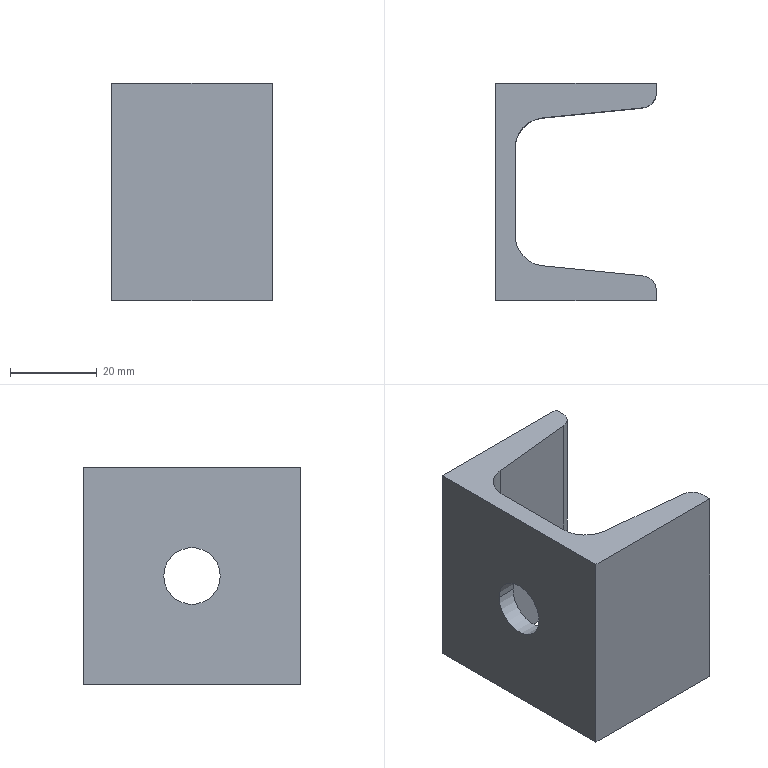Part | SolidWorks | features BaseBody 1 | 1 solid | 16 faces | box 37 x 50 x 50 mm | volume 34025 mm3 | plane 10 | cylinder 6 | commonest cylinder face diameters 7 x2 13 x2 14 x2
STEP:
#1=CARTESIAN_POINT('',(-13.5,-6.5,25.));
#2=VERTEX_POINT('',#1);
#3=CARTESIAN_POINT('',(-13.5,6.5,25.));
#4=VERTEX_POINT('',#3);
#5=CARTESIAN_POINT('',(-13.5,0.,25.));
#6=DIRECTION('',(1.,0.,0.));
#7=DIRECTION('',(0.,1.,0.));
#8=AXIS2_PLACEMENT_3D('',#5,#6,#7);
#9=CIRCLE('',#8,6.5);
#10=EDGE_CURVE('',#2,#4,#9,.T.);
#11=ORIENTED_EDGE('',*,*,#10,.F.);
#12=CARTESIAN_POINT('',(-9.,-6.5,25.));
#13=VERTEX_POINT('',#12);
#14=CARTESIAN_POINT('',(-13.5,-6.5,25.));
#15=DIRECTION('',(1.,0.,0.));
#16=VECTOR('',#15,1000.);
#17=LINE('',#14,#16);
#18=EDGE_CURVE('',#2,#13,#17,.T.);
#19=ORIENTED_EDGE('',*,*,#18,.T.);
#20=CARTESIAN_POINT('',(-9.,6.5,25.));
#21=VERTEX_POINT('',#20);
#22=CARTESIAN_POINT('',(-9.,0.,25.));
#23=DIRECTION('',(-1.,0.,0.));
#24=DIRECTION('',(0.,1.,0.));
#25=AXIS2_PLACEMENT_3D('',#22,#23,#24);
#26=CIRCLE('',#25,6.5);
#27=EDGE_CURVE('',#21,#13,#26,.T.);
#28=ORIENTED_EDGE('',*,*,#27,.F.);
#29=CARTESIAN_POINT('',(-13.5,6.5,25.));
#30=DIRECTION('',(1.,0.,0.));
#31=VECTOR('',#30,1000.);
#32=LINE('',#29,#31);
#33=EDGE_CURVE('',#4,#21,#32,.T.);
#34=ORIENTED_EDGE('',*,*,#33,.F.);
#35=EDGE_LOOP('',(#11,#19,#28,#34));
#36=FACE_OUTER_BOUND('',#35,.T.);
#37=CARTESIAN_POINT('',(-13.5,0.,25.));
#38=DIRECTION('',(1.,0.,0.));
#39=DIRECTION('',(0.,1.,0.));
#40=AXIS2_PLACEMENT_3D('',#37,#38,#39);
#41=CYLINDRICAL_SURFACE('',#40,6.5);
#42=ADVANCED_FACE('',(#36),#41,.F.);
#43=CARTESIAN_POINT('',(-13.5,0.,25.));
#44=DIRECTION('',(1.,0.,0.));
#45=DIRECTION('',(0.,1.,0.));
#46=AXIS2_PLACEMENT_3D('',#43,#44,#45);
#47=CIRCLE('',#46,6.5);
#48=EDGE_CURVE('',#4,#2,#47,.T.);
#49=ORIENTED_EDGE('',*,*,#48,.T.);
#50=ORIENTED_EDGE('',*,*,#10,.T.);
#51=EDGE_LOOP('',(#49,#50));
#52=FACE_BOUND('',#51,.T.);
#53=CARTESIAN_POINT('',(-13.5,25.,0.));
#54=VERTEX_POINT('',#53);
#55=CARTESIAN_POINT('',(-13.5,-25.,0.));
#56=VERTEX_POINT('',#55);
#57=CARTESIAN_POINT('',(-13.5,0.,0.));
#58=DIRECTION('',(0.,-1.,0.));
#59=VECTOR('',#58,1000.);
#60=LINE('',#57,#59);
#61=EDGE_CURVE('',#54,#56,#60,.T.);
#62=ORIENTED_EDGE('',*,*,#61,.T.);
#63=CARTESIAN_POINT('',(-13.5,-25.,50.));
#64=VERTEX_POINT('',#63);
#65=CARTESIAN_POINT('',(-13.5,-25.,0.));
#66=DIRECTION('',(0.,0.,1.));
#67=VECTOR('',#66,1000.);
#68=LINE('',#65,#67);
#69=EDGE_CURVE('',#56,#64,#68,.T.);
#70=ORIENTED_EDGE('',*,*,#69,.T.);
#71=CARTESIAN_POINT('',(-13.5,25.,50.));
#72=VERTEX_POINT('',#71);
#73=CARTESIAN_POINT('',(-13.5,0.,50.));
#74=DIRECTION('',(0.,1.,0.));
#75=VECTOR('',#74,1000.);
#76=LINE('',#73,#75);
#77=EDGE_CURVE('',#64,#72,#76,.T.);
#78=ORIENTED_EDGE('',*,*,#77,.T.);
#79=CARTESIAN_POINT('',(-13.5,25.,0.));
#80=DIRECTION('',(0.,0.,-1.));
#81=VECTOR('',#80,1000.);
#82=LINE('',#79,#81);
#83=EDGE_CURVE('',#72,#54,#82,.T.);
#84=ORIENTED_EDGE('',*,*,#83,.T.);
#85=EDGE_LOOP('',(#62,#70,#78,#84));
#86=FACE_OUTER_BOUND('',#85,.T.);
#87=CARTESIAN_POINT('',(-13.5,0.,0.));
#88=DIRECTION('',(-1.,0.,0.));
#89=DIRECTION('',(0.,-1.,0.));
#90=AXIS2_PLACEMENT_3D('',#87,#88,#89);
#91=PLANE('',#90);
#92=ADVANCED_FACE('',(#52,#86),#91,.T.);
#93=ORIENTED_EDGE('',*,*,#18,.F.);
#94=ORIENTED_EDGE('',*,*,#48,.F.);
#95=ORIENTED_EDGE('',*,*,#33,.T.);
#96=CARTESIAN_POINT('',(-9.,0.,25.));
#97=DIRECTION('',(-1.,0.,0.));
#98=DIRECTION('',(0.,1.,0.));
#99=AXIS2_PLACEMENT_3D('',#96,#97,#98);
#100=CIRCLE('',#99,6.5);
#101=EDGE_CURVE('',#13,#21,#100,.T.);
#102=ORIENTED_EDGE('',*,*,#101,.F.);
#103=EDGE_LOOP('',(#93,#94,#95,#102));
#104=FACE_OUTER_BOUND('',#103,.T.);
#105=CARTESIAN_POINT('',(-13.5,0.,25.));
#106=DIRECTION('',(1.,0.,0.));
#107=DIRECTION('',(0.,1.,0.));
#108=AXIS2_PLACEMENT_3D('',#105,#106,#107);
#109=CYLINDRICAL_SURFACE('',#108,6.5);
#110=ADVANCED_FACE('',(#104),#109,.F.);
#111=CARTESIAN_POINT('',(23.5,-25.,0.));
#112=VERTEX_POINT('',#111);
#113=CARTESIAN_POINT('',(23.5,-25.,0.));
#114=DIRECTION('',(1.,0.,0.));
#115=VECTOR('',#114,1000.);
#116=LINE('',#113,#115);
#117=EDGE_CURVE('',#56,#112,#116,.T.);
#118=ORIENTED_EDGE('',*,*,#117,.T.);
#119=CARTESIAN_POINT('',(23.5,-25.,50.));
#120=VERTEX_POINT('',#119);
#121=CARTESIAN_POINT('',(23.5,-25.,0.));
#122=DIRECTION('',(0.,0.,1.));
#123=VECTOR('',#122,1000.);
#124=LINE('',#121,#123);
#125=EDGE_CURVE('',#112,#120,#124,.T.);
#126=ORIENTED_EDGE('',*,*,#125,.T.);
#127=CARTESIAN_POINT('',(23.5,-25.,50.));
#128=DIRECTION('',(-1.,0.,0.));
#129=VECTOR('',#128,1000.);
#130=LINE('',#127,#129);
#131=EDGE_CURVE('',#120,#64,#130,.T.);
#132=ORIENTED_EDGE('',*,*,#131,.T.);
#133=ORIENTED_EDGE('',*,*,#69,.F.);
#134=EDGE_LOOP('',(#118,#126,#132,#133));
#135=FACE_OUTER_BOUND('',#134,.T.);
#136=CARTESIAN_POINT('',(23.5,-25.,0.));
#137=DIRECTION('',(0.,-1.,0.));
#138=DIRECTION('',(0.,0.,-1.));
#139=AXIS2_PLACEMENT_3D('',#136,#137,#138);
#140=PLANE('',#139);
#141=ADVANCED_FACE('',(#135),#140,.T.);
#142=CARTESIAN_POINT('',(23.5,22.792,0.));
#143=VERTEX_POINT('',#142);
#144=CARTESIAN_POINT('',(23.5,25.,0.));
#145=VERTEX_POINT('',#144);
#146=CARTESIAN_POINT('',(23.5,0.,0.));
#147=DIRECTION('',(0.,1.,0.));
#148=VECTOR('',#147,1000.);
#149=LINE('',#146,#148);
#150=EDGE_CURVE('',#143,#145,#149,.T.);
#151=ORIENTED_EDGE('',*,*,#150,.F.);
#152=CARTESIAN_POINT('',(20.348,19.31,0.));
#153=VERTEX_POINT('',#152);
#154=CARTESIAN_POINT('',(20.,22.792,0.));
#155=DIRECTION('',(0.,0.,1.));
#156=DIRECTION('',(1.,0.,0.));
#157=AXIS2_PLACEMENT_3D('',#154,#155,#156);
#158=CIRCLE('',#157,3.5);
#159=EDGE_CURVE('',#153,#143,#158,.T.);
#160=ORIENTED_EDGE('',*,*,#159,.F.);
#161=CARTESIAN_POINT('',(-2.697,17.005,0.));
#162=VERTEX_POINT('',#161);
#163=CARTESIAN_POINT('',(-2.697,17.005,0.));
#164=DIRECTION('',(0.995,0.0995,0.));
#165=VECTOR('',#164,1000.);
#166=LINE('',#163,#165);
#167=EDGE_CURVE('',#162,#153,#166,.T.);
#168=ORIENTED_EDGE('',*,*,#167,.F.);
#169=CARTESIAN_POINT('',(-9.,10.04,0.));
#170=VERTEX_POINT('',#169);
#171=CARTESIAN_POINT('',(-2.,10.04,0.));
#172=DIRECTION('',(0.,0.,-1.));
#173=DIRECTION('',(1.,0.,0.));
#174=AXIS2_PLACEMENT_3D('',#171,#172,#173);
#175=CIRCLE('',#174,7.);
#176=EDGE_CURVE('',#170,#162,#175,.T.);
#177=ORIENTED_EDGE('',*,*,#176,.F.);
#178=CARTESIAN_POINT('',(-9.,-10.04,0.));
#179=VERTEX_POINT('',#178);
#180=CARTESIAN_POINT('',(-9.,0.,0.));
#181=DIRECTION('',(0.,1.,0.));
#182=VECTOR('',#181,1000.);
#183=LINE('',#180,#182);
#184=EDGE_CURVE('',#179,#170,#183,.T.);
#185=ORIENTED_EDGE('',*,*,#184,.F.);
#186=CARTESIAN_POINT('',(-2.697,-17.005,0.));
#187=VERTEX_POINT('',#186);
#188=CARTESIAN_POINT('',(-2.,-10.04,0.));
#189=DIRECTION('',(0.,0.,-1.));
#190=DIRECTION('',(1.,0.,0.));
#191=AXIS2_PLACEMENT_3D('',#188,#189,#190);
#192=CIRCLE('',#191,7.);
#193=EDGE_CURVE('',#187,#179,#192,.T.);
#194=ORIENTED_EDGE('',*,*,#193,.F.);
#195=CARTESIAN_POINT('',(20.348,-19.31,0.));
#196=VERTEX_POINT('',#195);
#197=CARTESIAN_POINT('',(20.348,-19.31,0.));
#198=DIRECTION('',(-0.995,0.0995,0.));
#199=VECTOR('',#198,1000.);
#200=LINE('',#197,#199);
#201=EDGE_CURVE('',#196,#187,#200,.T.);
#202=ORIENTED_EDGE('',*,*,#201,.F.);
#203=CARTESIAN_POINT('',(23.5,-22.792,0.));
#204=VERTEX_POINT('',#203);
#205=CARTESIAN_POINT('',(20.,-22.792,0.));
#206=DIRECTION('',(0.,0.,1.));
#207=DIRECTION('',(1.,0.,0.));
#208=AXIS2_PLACEMENT_3D('',#205,#206,#207);
#209=CIRCLE('',#208,3.5);
#210=EDGE_CURVE('',#204,#196,#209,.T.);
#211=ORIENTED_EDGE('',*,*,#210,.F.);
#212=CARTESIAN_POINT('',(23.5,0.,0.));
#213=DIRECTION('',(0.,1.,0.));
#214=VECTOR('',#213,1000.);
#215=LINE('',#212,#214);
#216=EDGE_CURVE('',#112,#204,#215,.T.);
#217=ORIENTED_EDGE('',*,*,#216,.F.);
#218=ORIENTED_EDGE('',*,*,#117,.F.);
#219=ORIENTED_EDGE('',*,*,#61,.F.);
#220=CARTESIAN_POINT('',(5.,25.,0.));
#221=DIRECTION('',(-1.,0.,0.));
#222=VECTOR('',#221,1000.);
#223=LINE('',#220,#222);
#224=EDGE_CURVE('',#145,#54,#223,.T.);
#225=ORIENTED_EDGE('',*,*,#224,.F.);
#226=EDGE_LOOP('',(#151,#160,#168,#177,#185,#194,#202,#211,#217,#218,#219,#225));
#227=FACE_OUTER_BOUND('',#226,.T.);
#228=CARTESIAN_POINT('',(5.,0.,0.));
#229=DIRECTION('',(0.,0.,1.));
#230=DIRECTION('',(1.,0.,0.));
#231=AXIS2_PLACEMENT_3D('',#228,#229,#230);
#232=PLANE('',#231);
#233=ADVANCED_FACE('',(#227),#232,.F.);
#234=ORIENTED_EDGE('',*,*,#224,.T.);
#235=ORIENTED_EDGE('',*,*,#83,.F.);
#236=CARTESIAN_POINT('',(23.5,25.,50.));
#237=VERTEX_POINT('',#236);
#238=CARTESIAN_POINT('',(-13.5,25.,50.));
#239=DIRECTION('',(1.,0.,0.));
#240=VECTOR('',#239,1000.);
#241=LINE('',#238,#240);
#242=EDGE_CURVE('',#72,#237,#241,.T.);
#243=ORIENTED_EDGE('',*,*,#242,.T.);
#244=CARTESIAN_POINT('',(23.5,25.,0.));
#245=DIRECTION('',(0.,0.,-1.));
#246=VECTOR('',#245,1000.);
#247=LINE('',#244,#246);
#248=EDGE_CURVE('',#237,#145,#247,.T.);
#249=ORIENTED_EDGE('',*,*,#248,.T.);
#250=EDGE_LOOP('',(#234,#235,#243,#249));
#251=FACE_OUTER_BOUND('',#250,.T.);
#252=CARTESIAN_POINT('',(-13.5,25.,0.));
#253=DIRECTION('',(0.,1.,0.));
#254=DIRECTION('',(-1.,0.,0.));
#255=AXIS2_PLACEMENT_3D('',#252,#253,#254);
#256=PLANE('',#255);
#257=ADVANCED_FACE('',(#251),#256,.T.);
#258=CARTESIAN_POINT('',(20.348,19.31,50.));
#259=VERTEX_POINT('',#258);
#260=CARTESIAN_POINT('',(23.5,22.792,50.));
#261=VERTEX_POINT('',#260);
#262=CARTESIAN_POINT('',(20.,22.792,50.));
#263=DIRECTION('',(0.,0.,1.));
#264=DIRECTION('',(1.,0.,0.));
#265=AXIS2_PLACEMENT_3D('',#262,#263,#264);
#266=CIRCLE('',#265,3.5);
#267=EDGE_CURVE('',#259,#261,#266,.T.);
#268=ORIENTED_EDGE('',*,*,#267,.T.);
#269=CARTESIAN_POINT('',(23.5,0.,50.));
#270=DIRECTION('',(0.,1.,0.));
#271=VECTOR('',#270,1000.);
#272=LINE('',#269,#271);
#273=EDGE_CURVE('',#261,#237,#272,.T.);
#274=ORIENTED_EDGE('',*,*,#273,.T.);
#275=ORIENTED_EDGE('',*,*,#242,.F.);
#276=ORIENTED_EDGE('',*,*,#77,.F.);
#277=ORIENTED_EDGE('',*,*,#131,.F.);
#278=CARTESIAN_POINT('',(23.5,-22.792,50.));
#279=VERTEX_POINT('',#278);
#280=CARTESIAN_POINT('',(23.5,0.,50.));
#281=DIRECTION('',(0.,1.,0.));
#282=VECTOR('',#281,1000.);
#283=LINE('',#280,#282);
#284=EDGE_CURVE('',#120,#279,#283,.T.);
#285=ORIENTED_EDGE('',*,*,#284,.T.);
#286=CARTESIAN_POINT('',(20.348,-19.31,50.));
#287=VERTEX_POINT('',#286);
#288=CARTESIAN_POINT('',(20.,-22.792,50.));
#289=DIRECTION('',(0.,0.,1.));
#290=DIRECTION('',(1.,0.,0.));
#291=AXIS2_PLACEMENT_3D('',#288,#289,#290);
#292=CIRCLE('',#291,3.5);
#293=EDGE_CURVE('',#279,#287,#292,.T.);
#294=ORIENTED_EDGE('',*,*,#293,.T.);
#295=CARTESIAN_POINT('',(-2.697,-17.005,50.));
#296=VERTEX_POINT('',#295);
#297=CARTESIAN_POINT('',(20.348,-19.31,50.));
#298=DIRECTION('',(-0.995,0.0995,0.));
#299=VECTOR('',#298,1000.);
#300=LINE('',#297,#299);
#301=EDGE_CURVE('',#287,#296,#300,.T.);
#302=ORIENTED_EDGE('',*,*,#301,.T.);
#303=CARTESIAN_POINT('',(-9.,-10.04,50.));
#304=VERTEX_POINT('',#303);
#305=CARTESIAN_POINT('',(-2.,-10.04,50.));
#306=DIRECTION('',(0.,0.,-1.));
#307=DIRECTION('',(1.,0.,0.));
#308=AXIS2_PLACEMENT_3D('',#305,#306,#307);
#309=CIRCLE('',#308,7.);
#310=EDGE_CURVE('',#296,#304,#309,.T.);
#311=ORIENTED_EDGE('',*,*,#310,.T.);
#312=CARTESIAN_POINT('',(-9.,10.04,50.));
#313=VERTEX_POINT('',#312);
#314=CARTESIAN_POINT('',(-9.,0.,50.));
#315=DIRECTION('',(0.,1.,0.));
#316=VECTOR('',#315,1000.);
#317=LINE('',#314,#316);
#318=EDGE_CURVE('',#304,#313,#317,.T.);
#319=ORIENTED_EDGE('',*,*,#318,.T.);
#320=CARTESIAN_POINT('',(-2.697,17.005,50.));
#321=VERTEX_POINT('',#320);
#322=CARTESIAN_POINT('',(-2.,10.04,50.));
#323=DIRECTION('',(0.,0.,-1.));
#324=DIRECTION('',(1.,0.,0.));
#325=AXIS2_PLACEMENT_3D('',#322,#323,#324);
#326=CIRCLE('',#325,7.);
#327=EDGE_CURVE('',#313,#321,#326,.T.);
#328=ORIENTED_EDGE('',*,*,#327,.T.);
#329=CARTESIAN_POINT('',(-2.697,17.005,50.));
#330=DIRECTION('',(0.995,0.0995,0.));
#331=VECTOR('',#330,1000.);
#332=LINE('',#329,#331);
#333=EDGE_CURVE('',#321,#259,#332,.T.);
#334=ORIENTED_EDGE('',*,*,#333,.T.);
#335=EDGE_LOOP('',(#268,#274,#275,#276,#277,#285,#294,#302,#311,#319,#328,#334));
#336=FACE_OUTER_BOUND('',#335,.T.);
#337=CARTESIAN_POINT('',(5.,0.,50.));
#338=DIRECTION('',(0.,0.,1.));
#339=DIRECTION('',(1.,0.,0.));
#340=AXIS2_PLACEMENT_3D('',#337,#338,#339);
#341=PLANE('',#340);
#342=ADVANCED_FACE('',(#336),#341,.T.);
#343=ORIENTED_EDGE('',*,*,#27,.T.);
#344=ORIENTED_EDGE('',*,*,#101,.T.);
#345=EDGE_LOOP('',(#343,#344));
#346=FACE_BOUND('',#345,.T.);
#347=ORIENTED_EDGE('',*,*,#184,.T.);
#348=CARTESIAN_POINT('',(-9.,10.04,0.));
#349=DIRECTION('',(0.,0.,1.));
#350=VECTOR('',#349,1000.);
#351=LINE('',#348,#350);
#352=EDGE_CURVE('',#170,#313,#351,.T.);
#353=ORIENTED_EDGE('',*,*,#352,.T.);
#354=ORIENTED_EDGE('',*,*,#318,.F.);
#355=CARTESIAN_POINT('',(-9.,-10.04,0.));
#356=DIRECTION('',(0.,0.,-1.));
#357=VECTOR('',#356,1000.);
#358=LINE('',#355,#357);
#359=EDGE_CURVE('',#304,#179,#358,.T.);
#360=ORIENTED_EDGE('',*,*,#359,.T.);
#361=EDGE_LOOP('',(#347,#353,#354,#360));
#362=FACE_OUTER_BOUND('',#361,.T.);
#363=CARTESIAN_POINT('',(-9.,0.,0.));
#364=DIRECTION('',(1.,0.,0.));
#365=DIRECTION('',(0.,0.,-1.));
#366=AXIS2_PLACEMENT_3D('',#363,#364,#365);
#367=PLANE('',#366);
#368=ADVANCED_FACE('',(#346,#362),#367,.T.);
#369=ORIENTED_EDGE('',*,*,#216,.T.);
#370=CARTESIAN_POINT('',(23.5,-22.792,0.));
#371=DIRECTION('',(0.,0.,1.));
#372=VECTOR('',#371,1000.);
#373=LINE('',#370,#372);
#374=EDGE_CURVE('',#204,#279,#373,.T.);
#375=ORIENTED_EDGE('',*,*,#374,.T.);
#376=ORIENTED_EDGE('',*,*,#284,.F.);
#377=ORIENTED_EDGE('',*,*,#125,.F.);
#378=EDGE_LOOP('',(#369,#375,#376,#377));
#379=FACE_OUTER_BOUND('',#378,.T.);
#380=CARTESIAN_POINT('',(23.5,-22.792,0.));
#381=DIRECTION('',(1.,0.,0.));
#382=DIRECTION('',(0.,0.,-1.));
#383=AXIS2_PLACEMENT_3D('',#380,#381,#382);
#384=PLANE('',#383);
#385=ADVANCED_FACE('',(#379),#384,.T.);
#386=ORIENTED_EDGE('',*,*,#150,.T.);
#387=ORIENTED_EDGE('',*,*,#248,.F.);
#388=ORIENTED_EDGE('',*,*,#273,.F.);
#389=CARTESIAN_POINT('',(23.5,22.792,0.));
#390=DIRECTION('',(0.,0.,-1.));
#391=VECTOR('',#390,1000.);
#392=LINE('',#389,#391);
#393=EDGE_CURVE('',#261,#143,#392,.T.);
#394=ORIENTED_EDGE('',*,*,#393,.T.);
#395=EDGE_LOOP('',(#386,#387,#388,#394));
#396=FACE_OUTER_BOUND('',#395,.T.);
#397=CARTESIAN_POINT('',(23.5,25.,0.));
#398=DIRECTION('',(1.,0.,0.));
#399=DIRECTION('',(0.,0.,-1.));
#400=AXIS2_PLACEMENT_3D('',#397,#398,#399);
#401=PLANE('',#400);
#402=ADVANCED_FACE('',(#396),#401,.T.);
#403=ORIENTED_EDGE('',*,*,#159,.T.);
#404=ORIENTED_EDGE('',*,*,#393,.F.);
#405=ORIENTED_EDGE('',*,*,#267,.F.);
#406=CARTESIAN_POINT('',(20.348,19.31,0.));
#407=DIRECTION('',(0.,0.,-1.));
#408=VECTOR('',#407,1000.);
#409=LINE('',#406,#408);
#410=EDGE_CURVE('',#259,#153,#409,.T.);
#411=ORIENTED_EDGE('',*,*,#410,.T.);
#412=EDGE_LOOP('',(#403,#404,#405,#411));
#413=FACE_OUTER_BOUND('',#412,.T.);
#414=CARTESIAN_POINT('',(20.,22.792,0.));
#415=DIRECTION('',(0.,0.,1.));
#416=DIRECTION('',(1.,0.,0.));
#417=AXIS2_PLACEMENT_3D('',#414,#415,#416);
#418=CYLINDRICAL_SURFACE('',#417,3.5);
#419=ADVANCED_FACE('',(#413),#418,.T.);
#420=ORIENTED_EDGE('',*,*,#167,.T.);
#421=ORIENTED_EDGE('',*,*,#410,.F.);
#422=ORIENTED_EDGE('',*,*,#333,.F.);
#423=CARTESIAN_POINT('',(-2.697,17.005,0.));
#424=DIRECTION('',(0.,0.,-1.));
#425=VECTOR('',#424,1000.);
#426=LINE('',#423,#425);
#427=EDGE_CURVE('',#321,#162,#426,.T.);
#428=ORIENTED_EDGE('',*,*,#427,.T.);
#429=EDGE_LOOP('',(#420,#421,#422,#428));
#430=FACE_OUTER_BOUND('',#429,.T.);
#431=CARTESIAN_POINT('',(20.348,19.31,0.));
#432=DIRECTION('',(0.0995,-0.995,0.));
#433=DIRECTION('',(0.995,0.0995,0.));
#434=AXIS2_PLACEMENT_3D('',#431,#432,#433);
#435=PLANE('',#434);
#436=ADVANCED_FACE('',(#430),#435,.T.);
#437=ORIENTED_EDGE('',*,*,#352,.F.);
#438=ORIENTED_EDGE('',*,*,#176,.T.);
#439=ORIENTED_EDGE('',*,*,#427,.F.);
#440=ORIENTED_EDGE('',*,*,#327,.F.);
#441=EDGE_LOOP('',(#437,#438,#439,#440));
#442=FACE_OUTER_BOUND('',#441,.T.);
#443=CARTESIAN_POINT('',(-2.,10.04,0.));
#444=DIRECTION('',(0.,0.,1.));
#445=DIRECTION('',(1.,0.,0.));
#446=AXIS2_PLACEMENT_3D('',#443,#444,#445);
#447=CYLINDRICAL_SURFACE('',#446,7.);
#448=ADVANCED_FACE('',(#442),#447,.F.);
#449=CARTESIAN_POINT('',(-2.697,-17.005,0.));
#450=DIRECTION('',(0.,0.,1.));
#451=VECTOR('',#450,1000.);
#452=LINE('',#449,#451);
#453=EDGE_CURVE('',#187,#296,#452,.T.);
#454=ORIENTED_EDGE('',*,*,#453,.F.);
#455=ORIENTED_EDGE('',*,*,#193,.T.);
#456=ORIENTED_EDGE('',*,*,#359,.F.);
#457=ORIENTED_EDGE('',*,*,#310,.F.);
#458=EDGE_LOOP('',(#454,#455,#456,#457));
#459=FACE_OUTER_BOUND('',#458,.T.);
#460=CARTESIAN_POINT('',(-2.,-10.04,0.));
#461=DIRECTION('',(0.,0.,1.));
#462=DIRECTION('',(1.,0.,0.));
#463=AXIS2_PLACEMENT_3D('',#460,#461,#462);
#464=CYLINDRICAL_SURFACE('',#463,7.);
#465=ADVANCED_FACE('',(#459),#464,.F.);
#466=ORIENTED_EDGE('',*,*,#201,.T.);
#467=ORIENTED_EDGE('',*,*,#453,.T.);
#468=ORIENTED_EDGE('',*,*,#301,.F.);
#469=CARTESIAN_POINT('',(20.348,-19.31,0.));
#470=DIRECTION('',(0.,0.,-1.));
#471=VECTOR('',#470,1000.);
#472=LINE('',#469,#471);
#473=EDGE_CURVE('',#287,#196,#472,.T.);
#474=ORIENTED_EDGE('',*,*,#473,.T.);
#475=EDGE_LOOP('',(#466,#467,#468,#474));
#476=FACE_OUTER_BOUND('',#475,.T.);
#477=CARTESIAN_POINT('',(-2.697,-17.005,0.));
#478=DIRECTION('',(0.0995,0.995,0.));
#479=DIRECTION('',(-0.995,0.0995,0.));
#480=AXIS2_PLACEMENT_3D('',#477,#478,#479);
#481=PLANE('',#480);
#482=ADVANCED_FACE('',(#476),#481,.T.);
#483=ORIENTED_EDGE('',*,*,#210,.T.);
#484=ORIENTED_EDGE('',*,*,#473,.F.);
#485=ORIENTED_EDGE('',*,*,#293,.F.);
#486=ORIENTED_EDGE('',*,*,#374,.F.);
#487=EDGE_LOOP('',(#483,#484,#485,#486));
#488=FACE_OUTER_BOUND('',#487,.T.);
#489=CARTESIAN_POINT('',(20.,-22.792,0.));
#490=DIRECTION('',(0.,0.,1.));
#491=DIRECTION('',(1.,0.,0.));
#492=AXIS2_PLACEMENT_3D('',#489,#490,#491);
#493=CYLINDRICAL_SURFACE('',#492,3.5);
#494=ADVANCED_FACE('',(#488),#493,.T.);
#495=CLOSED_SHELL('',(#42,#92,#110,#141,#233,#257,#342,#368,#385,#402,#419,#436,#448,#465,#482,#494));
#496=MANIFOLD_SOLID_BREP('',#495);
#497=CARTESIAN_POINT('',(0.,0.,0.));
#498=DIRECTION('',(0.,0.,1.));
#499=DIRECTION('',(1.,0.,0.));
#500=AXIS2_PLACEMENT_3D('',#497,#498,#499);
#501=(LENGTH_UNIT()NAMED_UNIT(*)SI_UNIT(.MILLI.,.METRE.));
#502=UNCERTAINTY_MEASURE_WITH_UNIT(LENGTH_MEASURE(0.00001),#501,'','');
#503=(NAMED_UNIT(*)PLANE_ANGLE_UNIT()SI_UNIT($,.RADIAN.));
#504=(NAMED_UNIT(*)SI_UNIT($,.STERADIAN.)SOLID_ANGLE_UNIT());
#505=(GEOMETRIC_REPRESENTATION_CONTEXT(3)GLOBAL_UNCERTAINTY_ASSIGNED_CONTEXT((#502))GLOBAL_UNIT_ASSIGNED_CONTEXT((#501,#503,#504))REPRESENTATION_CONTEXT('',''));
#506=ADVANCED_BREP_SHAPE_REPRESENTATION('',(#496,#500),#505);